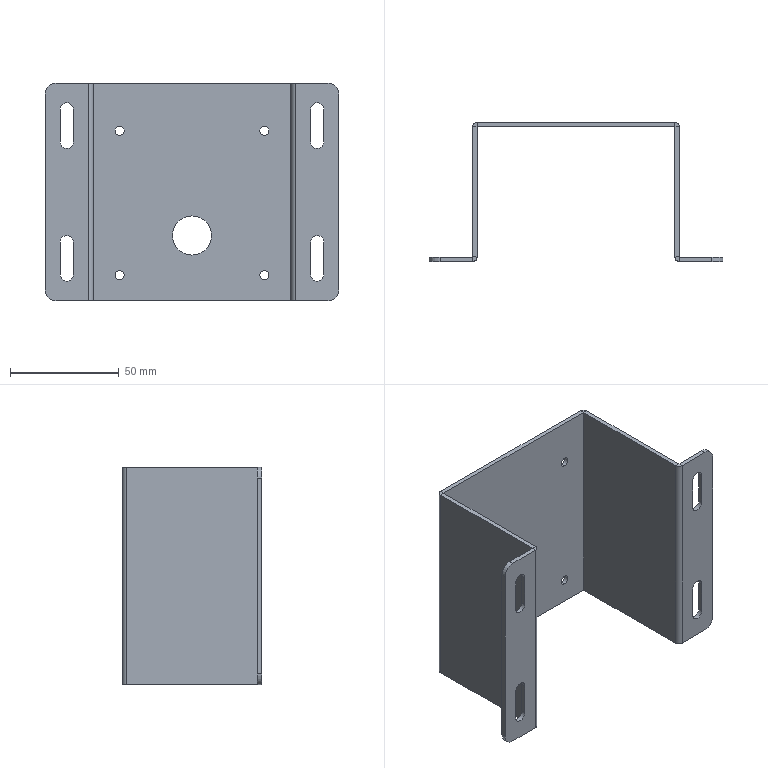Part | SolidWorks | features Cut 1, Fillet 1, FlatPattern 1, HoleWzd 1, ICE 1, SMBaseFlange 1, SheetMetal 1 | 1 solid | 72 faces | box 135 x 64 x 100 mm | volume 49813 mm3 | plane 38 | cylinder 34 | commonest cylinder face diameters 4.2 x12 6 x12 0.2 x4 10 x4 18 x2